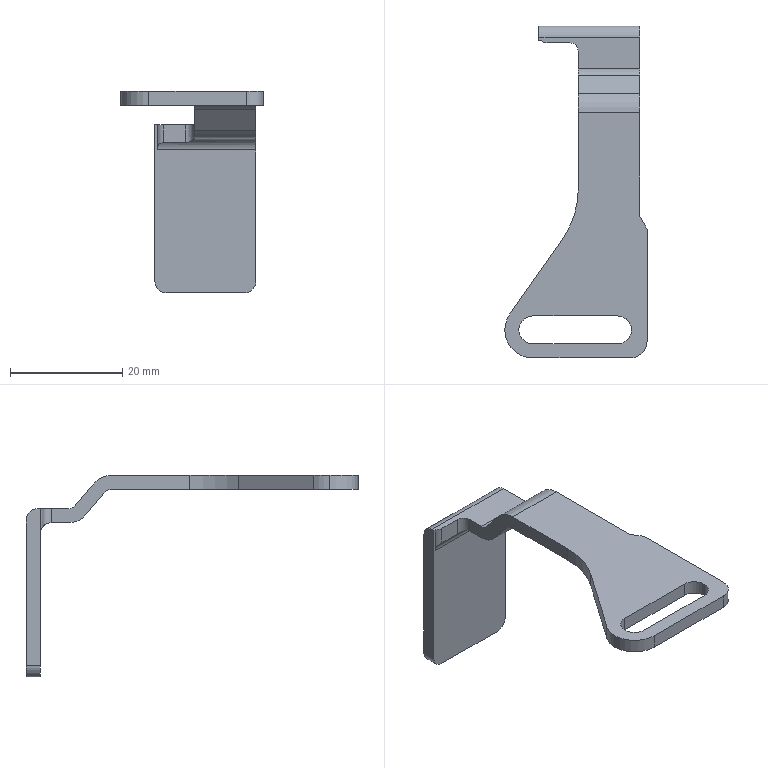Part | STEP file | JDC-75-2 | 1 solid | 36 faces | box 25.398 x 59.274 x 36 mm | volume 3330 mm3 | plane 19 | cylinder 17 | commonest cylinder face diameters 4 x5 3 x3 5 x3 10 x2 6 x1 8 x1